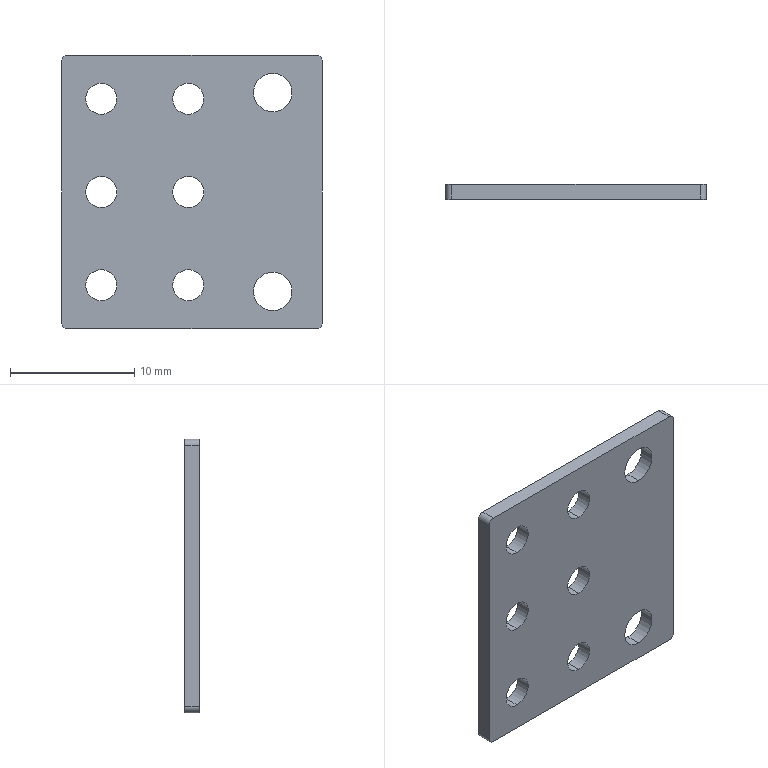Part | STEP file | 1 solid | 26 faces | box 21 x 1.2 x 22 mm | volume 500.685 mm3 | cylinder 20 | plane 6 | commonest cylinder face diameters 2.5 x12 1 x4 3.1 x4